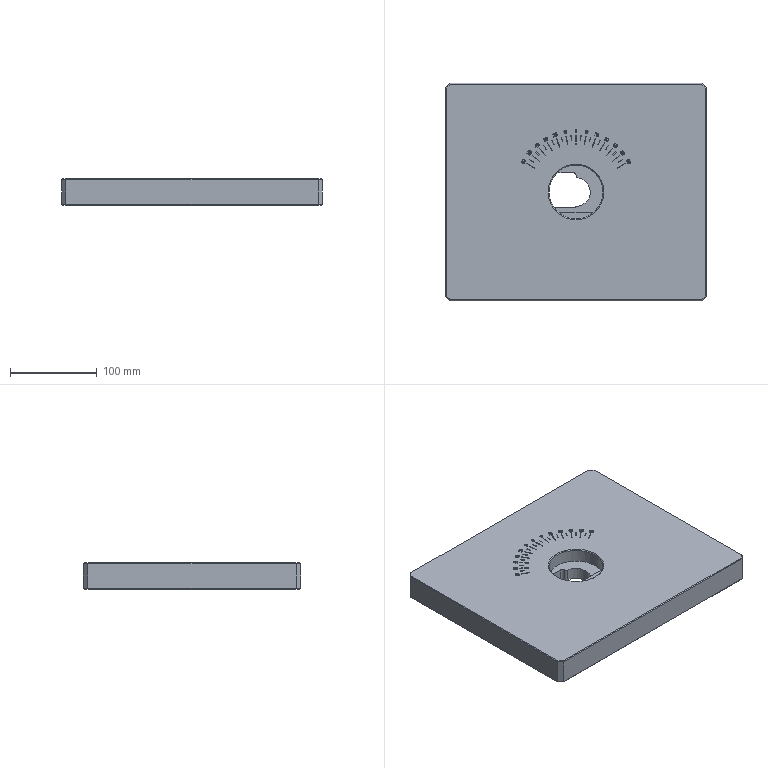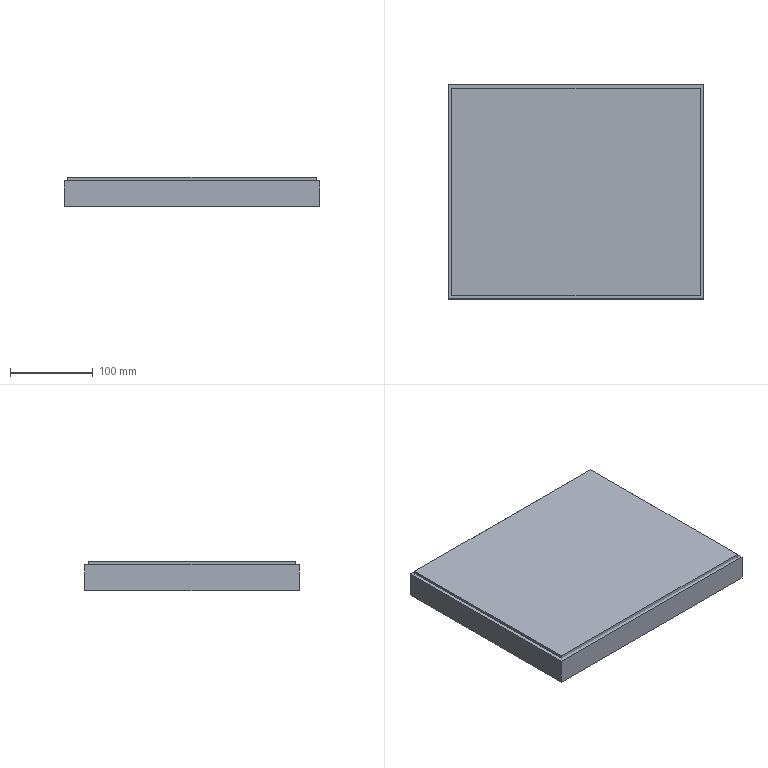CAM job | NX | 3-axis milling | part box 300 x 250 x 30 mm | stock box 308 x 258 x 35 mm
Tools:
number,name,description,diameter,corner_radius,flute_length,length,flutes
3,D63,Milling Tool-5 Parameters,63.0,0.0,50.0,75.0,2
4,D10,Milling Tool-5 Parameters,10.0,0.0,50.0,75.0,2
15,D4,Milling Tool-5 Parameters,4.0,0.0,50.0,75.0,2
5,D10JING,Milling Tool-5 Parameters,10.0,0.0,50.0,75.0,2
1,D6A45,Milling Tool-5 Parameters,6.0,0.0,3.0,3.0,2
13,R0.5,Milling Tool-5 Parameters,0.2,0.1,50.0,75.0,2
Operations:
program,operation,operation_type,tool,method,geometry_group,spindle_rpm,surface_speed,feed_per_tooth,feed_cut,feed_plunge,cut_length_mm,path_length_mm,cut_time_min,machine_time_min
1-305-255-35毛胚,FLOOR_WALL_COPY,VolumeBased25DMillingOperation,D63,METHOD,A,6500.0,1286.0,0.0962,1250.0,100.0,2414.785,2468.785,1.932,1.937
1-305-255-35毛胚,ADAPTIVE_MILLING_COPY,CavityMilling,D10,METHOD,A,9500.0,298.0,0.1842,3500.0,1000.0,19477.013,22915.516,7.209,7.553
1-305-255-35毛胚,ZLEVEL_PROFILE_1_COPY_COPY_COPY,ZLevelMilling,D10JING,METHOD,A,9500.0,298.0,0.0526,1000.0,100.0,169.31,233.31,0.1693,0.1757
1-305-255-35毛胚,ZLEVEL_PROFILE_1_COPY_COPY_COPY_COPY,ZLevelMilling,D10JING,METHOD,A,9500.0,298.0,0.0526,1000.0,100.0,165.626,255.626,0.1656,0.1746
1-305-255-35毛胚,ZLEVEL_PROFILE_1_COPY_COPY_COPY_COPY_COPY,ZLevelMilling,D10JING,METHOD,A,9500.0,298.0,0.0526,1000.0,100.0,118.95,236.95,0.1189,0.1307
1-305-255-35毛胚,FLOOR_WALL_1_COPY_1_COPY,VolumeBased25DMillingOperation,D10JING,METHOD,A,9500.0,298.0,0.0632,1200.0,1000.0,442.614,569.586,0.3703,0.3839
1-305-255-35毛胚,ZLEVEL_PROFILE_COPY_COPY_COPY_1_COPY,ZLevelMilling,D4,METHOD,A,9500.0,89.0,0.0789,1500.0,1000.0,936.824,2120.268,0.6865,0.8049
1-305-255-35毛胚,11_COPY_COPY_1_COPY_COPY,ZLevelMilling,D6A45,METHOD,A,9500.0,179.0,0.0526,1000.0,100.0,1302.113,1590.473,1.302,1.331
1-305-255-35毛胚,11_COPY_COPY_1_COPY_COPY_COPY,ZLevelMilling,D6A45,METHOD,A,9500.0,179.0,0.0526,1000.0,100.0,40.448,102.448,0.0404,0.0466
1-305-255-35毛胚,11_COPY_COPY_1_COPY_COPY_COPY_COPY,ZLevelMilling,D6A45,METHOD,A,9500.0,179.0,0.0526,1000.0,100.0,101.507,189.507,0.1015,0.1103
1-305-255-35毛胚,ZLEVEL_PROFILE_COPY_COPY_COPY_COPY_1,ZLevelMilling,R0.5,METHOD,A,9504.0,5.0,0.0631,1200.0,1000.0,2340.28,7081.566,1.964,2.438
2-305-255-35毛胚,FLOOR_WALL_COPY_COPY,VolumeBased25DMillingOperation,D63,METHOD,B,6500.0,1286.0,0.0962,1250.0,100.0,12073.995,13223.191,9.659,9.774
2-305-255-35毛胚,11_COPY_COPY_1_COPY_COPY_COPY_1,ZLevelMilling,D6A45,METHOD,B,9500.0,179.0,0.0526,1000.0,100.0,1100.469,1157.469,1.101,1.106
2-305-255-35毛胚,11_COPY_COPY_1_COPY_COPY_COPY_COPY_COPY,ZLevelMilling,D6A45,METHOD,B,9500.0,179.0,0.0526,1000.0,100.0,149.768,205.768,0.1498,0.1554